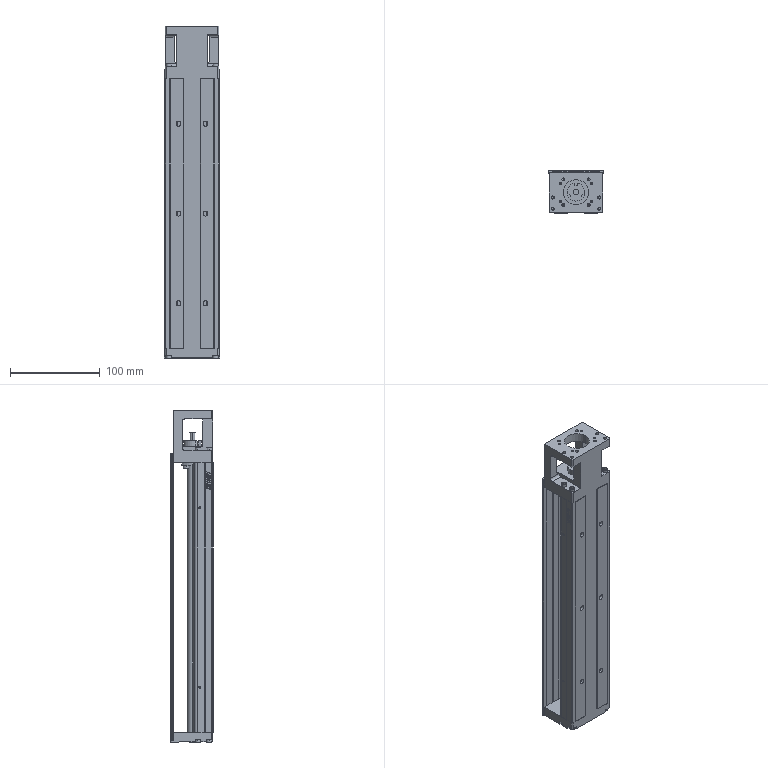Part | SolidWorks | features BaseBody 1 | 1 solid | 706 faces | box 62 x 47 x 370 mm | volume 387917 mm3 | plane 409 | cylinder 149 | spline 114 | cone 34 | commonest cylinder face diameters 5.5 x36 6 x31 2.459 x16 9.5 x12 1 x8 2.113 x8